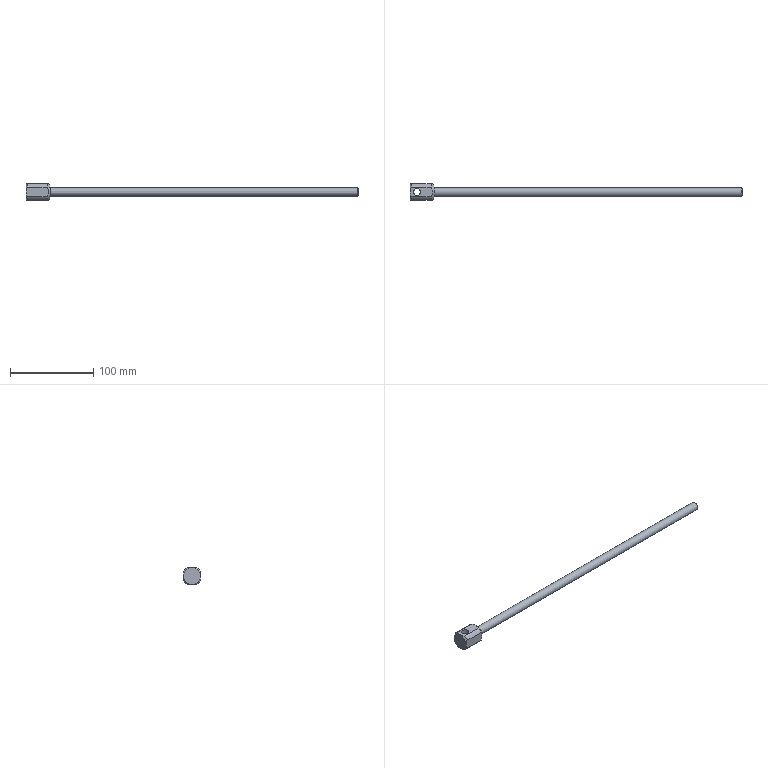Part | STEP file | GAS SHOCK A01S | 1 solid | 20 faces | box 398.5 x 20 x 20 mm | volume 38228 mm3 | plane 7 | cylinder 6 | cone 5 | torus 2 | commonest cylinder face diameters 23 x4 8.5 x1 10 x1